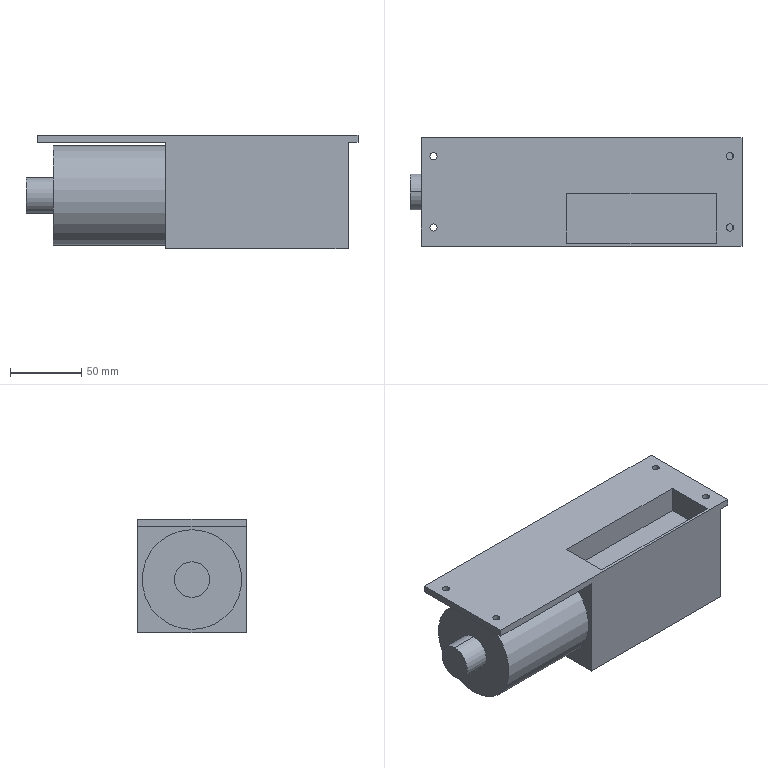Part | 1 solid | 33 faces | box 233 x 76 x 80 mm | volume 1016189 mm3 | plane 21 | cylinder 12 | commonest cylinder face diameters 5 x8 25 x2 70 x2
STEP:
#1=CARTESIAN_POINT('',(-120.5,0.,50.));
#2=VERTEX_POINT('',#1);
#3=CARTESIAN_POINT('',(-120.5,0.,25.));
#4=VERTEX_POINT('',#3);
#5=CARTESIAN_POINT('',(-120.5,0.,37.5));
#6=DIRECTION('',(-1.,0.,0.));
#7=DIRECTION('',(0.,0.,1.));
#8=AXIS2_PLACEMENT_3D('',#5,#6,#7);
#9=CIRCLE('',#8,12.5);
#10=EDGE_CURVE('',#2,#4,#9,.T.);
#11=ORIENTED_EDGE('',*,*,#10,.F.);
#12=CARTESIAN_POINT('',(-101.5,0.,50.));
#13=VERTEX_POINT('',#12);
#14=CARTESIAN_POINT('',(-120.5,0.,50.));
#15=DIRECTION('',(1.,0.,0.));
#16=VECTOR('',#15,1000.);
#17=LINE('',#14,#16);
#18=EDGE_CURVE('',#2,#13,#17,.T.);
#19=ORIENTED_EDGE('',*,*,#18,.T.);
#20=CARTESIAN_POINT('',(-101.5,0.,25.));
#21=VERTEX_POINT('',#20);
#22=CARTESIAN_POINT('',(-101.5,0.,37.5));
#23=DIRECTION('',(-1.,0.,0.));
#24=DIRECTION('',(0.,0.,1.));
#25=AXIS2_PLACEMENT_3D('',#22,#23,#24);
#26=CIRCLE('',#25,12.5);
#27=EDGE_CURVE('',#13,#21,#26,.T.);
#28=ORIENTED_EDGE('',*,*,#27,.T.);
#29=CARTESIAN_POINT('',(-120.5,0.,25.));
#30=DIRECTION('',(1.,0.,0.));
#31=VECTOR('',#30,1000.);
#32=LINE('',#29,#31);
#33=EDGE_CURVE('',#4,#21,#32,.T.);
#34=ORIENTED_EDGE('',*,*,#33,.F.);
#35=EDGE_LOOP('',(#11,#19,#28,#34));
#36=FACE_OUTER_BOUND('',#35,.T.);
#37=CARTESIAN_POINT('',(-120.5,0.,37.5));
#38=DIRECTION('',(1.,0.,0.));
#39=DIRECTION('',(0.,0.,-1.));
#40=AXIS2_PLACEMENT_3D('',#37,#38,#39);
#41=CYLINDRICAL_SURFACE('',#40,12.5);
#42=ADVANCED_FACE('',(#36),#41,.T.);
#43=CARTESIAN_POINT('',(-101.5,0.,72.5));
#44=VERTEX_POINT('',#43);
#45=CARTESIAN_POINT('',(-101.5,0.,2.5));
#46=VERTEX_POINT('',#45);
#47=CARTESIAN_POINT('',(-101.5,0.,37.5));
#48=DIRECTION('',(-1.,0.,0.));
#49=DIRECTION('',(0.,0.,1.));
#50=AXIS2_PLACEMENT_3D('',#47,#48,#49);
#51=CIRCLE('',#50,35.);
#52=EDGE_CURVE('',#44,#46,#51,.T.);
#53=ORIENTED_EDGE('',*,*,#52,.F.);
#54=CARTESIAN_POINT('',(-22.5,0.,72.5));
#55=VERTEX_POINT('',#54);
#56=CARTESIAN_POINT('',(-101.5,0.,72.5));
#57=DIRECTION('',(1.,0.,0.));
#58=VECTOR('',#57,1000.);
#59=LINE('',#56,#58);
#60=EDGE_CURVE('',#44,#55,#59,.T.);
#61=ORIENTED_EDGE('',*,*,#60,.T.);
#62=CARTESIAN_POINT('',(-22.5,0.,2.5));
#63=VERTEX_POINT('',#62);
#64=CARTESIAN_POINT('',(-22.5,0.,37.5));
#65=DIRECTION('',(-1.,0.,0.));
#66=DIRECTION('',(0.,0.,-1.));
#67=AXIS2_PLACEMENT_3D('',#64,#65,#66);
#68=CIRCLE('',#67,35.);
#69=EDGE_CURVE('',#55,#63,#68,.T.);
#70=ORIENTED_EDGE('',*,*,#69,.T.);
#71=CARTESIAN_POINT('',(-101.5,0.,2.5));
#72=DIRECTION('',(1.,0.,0.));
#73=VECTOR('',#72,1000.);
#74=LINE('',#71,#73);
#75=EDGE_CURVE('',#46,#63,#74,.T.);
#76=ORIENTED_EDGE('',*,*,#75,.F.);
#77=EDGE_LOOP('',(#53,#61,#70,#76));
#78=FACE_OUTER_BOUND('',#77,.T.);
#79=CARTESIAN_POINT('',(-101.5,0.,37.5));
#80=DIRECTION('',(1.,0.,0.));
#81=DIRECTION('',(0.,0.,-1.));
#82=AXIS2_PLACEMENT_3D('',#79,#80,#81);
#83=CYLINDRICAL_SURFACE('',#82,35.);
#84=ADVANCED_FACE('',(#78),#83,.T.);
#85=CARTESIAN_POINT('',(-106.5,25.,80.));
#86=VERTEX_POINT('',#85);
#87=CARTESIAN_POINT('',(-101.5,25.,80.));
#88=VERTEX_POINT('',#87);
#89=CARTESIAN_POINT('',(-104.,25.,80.));
#90=DIRECTION('',(0.,0.,1.));
#91=DIRECTION('',(1.,0.,0.));
#92=AXIS2_PLACEMENT_3D('',#89,#90,#91);
#93=CIRCLE('',#92,2.5);
#94=EDGE_CURVE('',#86,#88,#93,.T.);
#95=ORIENTED_EDGE('',*,*,#94,.T.);
#96=CARTESIAN_POINT('',(-101.5,25.,75.));
#97=VERTEX_POINT('',#96);
#98=CARTESIAN_POINT('',(-101.5,25.,90.));
#99=DIRECTION('',(0.,0.,-1.));
#100=VECTOR('',#99,1000.);
#101=LINE('',#98,#100);
#102=EDGE_CURVE('',#88,#97,#101,.T.);
#103=ORIENTED_EDGE('',*,*,#102,.T.);
#104=CARTESIAN_POINT('',(-106.5,25.,75.));
#105=VERTEX_POINT('',#104);
#106=CARTESIAN_POINT('',(-104.,25.,75.));
#107=DIRECTION('',(0.,0.,-1.));
#108=DIRECTION('',(-1.,0.,0.));
#109=AXIS2_PLACEMENT_3D('',#106,#107,#108);
#110=CIRCLE('',#109,2.5);
#111=EDGE_CURVE('',#97,#105,#110,.T.);
#112=ORIENTED_EDGE('',*,*,#111,.T.);
#113=CARTESIAN_POINT('',(-106.5,25.,90.));
#114=DIRECTION('',(0.,0.,-1.));
#115=VECTOR('',#114,1000.);
#116=LINE('',#113,#115);
#117=EDGE_CURVE('',#86,#105,#116,.T.);
#118=ORIENTED_EDGE('',*,*,#117,.F.);
#119=EDGE_LOOP('',(#95,#103,#112,#118));
#120=FACE_OUTER_BOUND('',#119,.T.);
#121=CARTESIAN_POINT('',(-104.,25.,90.));
#122=DIRECTION('',(0.,0.,-1.));
#123=DIRECTION('',(-1.,0.,0.));
#124=AXIS2_PLACEMENT_3D('',#121,#122,#123);
#125=CYLINDRICAL_SURFACE('',#124,2.5);
#126=ADVANCED_FACE('',(#120),#125,.F.);
#127=CARTESIAN_POINT('',(-106.5,-25.,80.));
#128=VERTEX_POINT('',#127);
#129=CARTESIAN_POINT('',(-101.5,-25.,80.));
#130=VERTEX_POINT('',#129);
#131=CARTESIAN_POINT('',(-104.,-25.,80.));
#132=DIRECTION('',(0.,0.,1.));
#133=DIRECTION('',(1.,0.,0.));
#134=AXIS2_PLACEMENT_3D('',#131,#132,#133);
#135=CIRCLE('',#134,2.5);
#136=EDGE_CURVE('',#128,#130,#135,.T.);
#137=ORIENTED_EDGE('',*,*,#136,.T.);
#138=CARTESIAN_POINT('',(-101.5,-25.,75.));
#139=VERTEX_POINT('',#138);
#140=CARTESIAN_POINT('',(-101.5,-25.,90.));
#141=DIRECTION('',(0.,0.,-1.));
#142=VECTOR('',#141,1000.);
#143=LINE('',#140,#142);
#144=EDGE_CURVE('',#130,#139,#143,.T.);
#145=ORIENTED_EDGE('',*,*,#144,.T.);
#146=CARTESIAN_POINT('',(-106.5,-25.,75.));
#147=VERTEX_POINT('',#146);
#148=CARTESIAN_POINT('',(-104.,-25.,75.));
#149=DIRECTION('',(0.,0.,-1.));
#150=DIRECTION('',(-1.,0.,0.));
#151=AXIS2_PLACEMENT_3D('',#148,#149,#150);
#152=CIRCLE('',#151,2.5);
#153=EDGE_CURVE('',#139,#147,#152,.T.);
#154=ORIENTED_EDGE('',*,*,#153,.T.);
#155=CARTESIAN_POINT('',(-106.5,-25.,90.));
#156=DIRECTION('',(0.,0.,-1.));
#157=VECTOR('',#156,1000.);
#158=LINE('',#155,#157);
#159=EDGE_CURVE('',#128,#147,#158,.T.);
#160=ORIENTED_EDGE('',*,*,#159,.F.);
#161=EDGE_LOOP('',(#137,#145,#154,#160));
#162=FACE_OUTER_BOUND('',#161,.T.);
#163=CARTESIAN_POINT('',(-104.,-25.,90.));
#164=DIRECTION('',(0.,0.,-1.));
#165=DIRECTION('',(-1.,0.,0.));
#166=AXIS2_PLACEMENT_3D('',#163,#164,#165);
#167=CYLINDRICAL_SURFACE('',#166,2.5);
#168=ADVANCED_FACE('',(#162),#167,.F.);
#169=CARTESIAN_POINT('',(101.5,-25.,80.));
#170=VERTEX_POINT('',#169);
#171=CARTESIAN_POINT('',(106.5,-25.,80.));
#172=VERTEX_POINT('',#171);
#173=CARTESIAN_POINT('',(104.,-25.,80.));
#174=DIRECTION('',(0.,0.,1.));
#175=DIRECTION('',(1.,0.,0.));
#176=AXIS2_PLACEMENT_3D('',#173,#174,#175);
#177=CIRCLE('',#176,2.5);
#178=EDGE_CURVE('',#170,#172,#177,.T.);
#179=ORIENTED_EDGE('',*,*,#178,.T.);
#180=CARTESIAN_POINT('',(106.5,-25.,75.));
#181=VERTEX_POINT('',#180);
#182=CARTESIAN_POINT('',(106.5,-25.,90.));
#183=DIRECTION('',(0.,0.,-1.));
#184=VECTOR('',#183,1000.);
#185=LINE('',#182,#184);
#186=EDGE_CURVE('',#172,#181,#185,.T.);
#187=ORIENTED_EDGE('',*,*,#186,.T.);
#188=CARTESIAN_POINT('',(101.5,-25.,75.));
#189=VERTEX_POINT('',#188);
#190=CARTESIAN_POINT('',(104.,-25.,75.));
#191=DIRECTION('',(0.,0.,-1.));
#192=DIRECTION('',(-1.,0.,0.));
#193=AXIS2_PLACEMENT_3D('',#190,#191,#192);
#194=CIRCLE('',#193,2.5);
#195=EDGE_CURVE('',#181,#189,#194,.T.);
#196=ORIENTED_EDGE('',*,*,#195,.T.);
#197=CARTESIAN_POINT('',(101.5,-25.,90.));
#198=DIRECTION('',(0.,0.,-1.));
#199=VECTOR('',#198,1000.);
#200=LINE('',#197,#199);
#201=EDGE_CURVE('',#170,#189,#200,.T.);
#202=ORIENTED_EDGE('',*,*,#201,.F.);
#203=EDGE_LOOP('',(#179,#187,#196,#202));
#204=FACE_OUTER_BOUND('',#203,.T.);
#205=CARTESIAN_POINT('',(104.,-25.,90.));
#206=DIRECTION('',(0.,0.,-1.));
#207=DIRECTION('',(-1.,0.,0.));
#208=AXIS2_PLACEMENT_3D('',#205,#206,#207);
#209=CYLINDRICAL_SURFACE('',#208,2.5);
#210=ADVANCED_FACE('',(#204),#209,.F.);
#211=CARTESIAN_POINT('',(101.5,25.,80.));
#212=VERTEX_POINT('',#211);
#213=CARTESIAN_POINT('',(106.5,25.,80.));
#214=VERTEX_POINT('',#213);
#215=CARTESIAN_POINT('',(104.,25.,80.));
#216=DIRECTION('',(0.,0.,1.));
#217=DIRECTION('',(1.,0.,0.));
#218=AXIS2_PLACEMENT_3D('',#215,#216,#217);
#219=CIRCLE('',#218,2.5);
#220=EDGE_CURVE('',#212,#214,#219,.T.);
#221=ORIENTED_EDGE('',*,*,#220,.T.);
#222=CARTESIAN_POINT('',(106.5,25.,75.));
#223=VERTEX_POINT('',#222);
#224=CARTESIAN_POINT('',(106.5,25.,90.));
#225=DIRECTION('',(0.,0.,-1.));
#226=VECTOR('',#225,1000.);
#227=LINE('',#224,#226);
#228=EDGE_CURVE('',#214,#223,#227,.T.);
#229=ORIENTED_EDGE('',*,*,#228,.T.);
#230=CARTESIAN_POINT('',(101.5,25.,75.));
#231=VERTEX_POINT('',#230);
#232=CARTESIAN_POINT('',(104.,25.,75.));
#233=DIRECTION('',(0.,0.,-1.));
#234=DIRECTION('',(-1.,0.,0.));
#235=AXIS2_PLACEMENT_3D('',#232,#233,#234);
#236=CIRCLE('',#235,2.5);
#237=EDGE_CURVE('',#223,#231,#236,.T.);
#238=ORIENTED_EDGE('',*,*,#237,.T.);
#239=CARTESIAN_POINT('',(101.5,25.,90.));
#240=DIRECTION('',(0.,0.,-1.));
#241=VECTOR('',#240,1000.);
#242=LINE('',#239,#241);
#243=EDGE_CURVE('',#212,#231,#242,.T.);
#244=ORIENTED_EDGE('',*,*,#243,.F.);
#245=EDGE_LOOP('',(#221,#229,#238,#244));
#246=FACE_OUTER_BOUND('',#245,.T.);
#247=CARTESIAN_POINT('',(104.,25.,90.));
#248=DIRECTION('',(0.,0.,-1.));
#249=DIRECTION('',(-1.,0.,0.));
#250=AXIS2_PLACEMENT_3D('',#247,#248,#249);
#251=CYLINDRICAL_SURFACE('',#250,2.5);
#252=ADVANCED_FACE('',(#246),#251,.F.);
#253=CARTESIAN_POINT('',(104.,-25.,75.));
#254=DIRECTION('',(0.,0.,-1.));
#255=DIRECTION('',(-1.,0.,0.));
#256=AXIS2_PLACEMENT_3D('',#253,#254,#255);
#257=CIRCLE('',#256,2.5);
#258=EDGE_CURVE('',#189,#181,#257,.T.);
#259=ORIENTED_EDGE('',*,*,#258,.F.);
#260=ORIENTED_EDGE('',*,*,#195,.F.);
#261=EDGE_LOOP('',(#259,#260));
#262=FACE_BOUND('',#261,.T.);
#263=CARTESIAN_POINT('',(104.,25.,75.));
#264=DIRECTION('',(0.,0.,-1.));
#265=DIRECTION('',(-1.,0.,0.));
#266=AXIS2_PLACEMENT_3D('',#263,#264,#265);
#267=CIRCLE('',#266,2.5);
#268=EDGE_CURVE('',#231,#223,#267,.T.);
#269=ORIENTED_EDGE('',*,*,#268,.F.);
#270=ORIENTED_EDGE('',*,*,#237,.F.);
#271=EDGE_LOOP('',(#269,#270));
#272=FACE_BOUND('',#271,.T.);
#273=CARTESIAN_POINT('',(105.5,-36.,75.));
#274=VERTEX_POINT('',#273);
#275=CARTESIAN_POINT('',(97.5,-36.,75.));
#276=VERTEX_POINT('',#275);
#277=CARTESIAN_POINT('',(105.5,-36.,75.));
#278=DIRECTION('',(-1.,0.,0.));
#279=VECTOR('',#278,1000.);
#280=LINE('',#277,#279);
#281=EDGE_CURVE('',#274,#276,#280,.T.);
#282=ORIENTED_EDGE('',*,*,#281,.T.);
#283=CARTESIAN_POINT('',(97.5,36.,75.));
#284=VERTEX_POINT('',#283);
#285=CARTESIAN_POINT('',(97.5,38.,75.));
#286=DIRECTION('',(0.,-1.,0.));
#287=VECTOR('',#286,1000.);
#288=LINE('',#285,#287);
#289=EDGE_CURVE('',#284,#276,#288,.T.);
#290=ORIENTED_EDGE('',*,*,#289,.F.);
#291=CARTESIAN_POINT('',(105.5,36.,75.));
#292=VERTEX_POINT('',#291);
#293=CARTESIAN_POINT('',(105.5,36.,75.));
#294=DIRECTION('',(-1.,0.,0.));
#295=VECTOR('',#294,1000.);
#296=LINE('',#293,#295);
#297=EDGE_CURVE('',#292,#284,#296,.T.);
#298=ORIENTED_EDGE('',*,*,#297,.F.);
#299=CARTESIAN_POINT('',(105.5,38.,75.));
#300=VERTEX_POINT('',#299);
#301=CARTESIAN_POINT('',(105.5,38.,75.));
#302=DIRECTION('',(0.,-1.,0.));
#303=VECTOR('',#302,1000.);
#304=LINE('',#301,#303);
#305=EDGE_CURVE('',#300,#292,#304,.T.);
#306=ORIENTED_EDGE('',*,*,#305,.F.);
#307=CARTESIAN_POINT('',(112.5,38.,75.));
#308=VERTEX_POINT('',#307);
#309=CARTESIAN_POINT('',(97.5,38.,75.));
#310=DIRECTION('',(1.,0.,0.));
#311=VECTOR('',#310,1000.);
#312=LINE('',#309,#311);
#313=EDGE_CURVE('',#300,#308,#312,.T.);
#314=ORIENTED_EDGE('',*,*,#313,.T.);
#315=CARTESIAN_POINT('',(112.5,-38.,75.));
#316=VERTEX_POINT('',#315);
#317=CARTESIAN_POINT('',(112.5,38.,75.));
#318=DIRECTION('',(0.,-1.,0.));
#319=VECTOR('',#318,1000.);
#320=LINE('',#317,#319);
#321=EDGE_CURVE('',#308,#316,#320,.T.);
#322=ORIENTED_EDGE('',*,*,#321,.T.);
#323=CARTESIAN_POINT('',(105.5,-38.,75.));
#324=VERTEX_POINT('',#323);
#325=CARTESIAN_POINT('',(97.5,-38.,75.));
#326=DIRECTION('',(1.,0.,0.));
#327=VECTOR('',#326,1000.);
#328=LINE('',#325,#327);
#329=EDGE_CURVE('',#324,#316,#328,.T.);
#330=ORIENTED_EDGE('',*,*,#329,.F.);
#331=CARTESIAN_POINT('',(105.5,-38.,75.));
#332=DIRECTION('',(0.,-1.,0.));
#333=VECTOR('',#332,1000.);
#334=LINE('',#331,#333);
#335=EDGE_CURVE('',#274,#324,#334,.T.);
#336=ORIENTED_EDGE('',*,*,#335,.F.);
#337=EDGE_LOOP('',(#282,#290,#298,#306,#314,#322,#330,#336));
#338=FACE_OUTER_BOUND('',#337,.T.);
#339=CARTESIAN_POINT('',(97.5,38.,75.));
#340=DIRECTION('',(0.,0.,1.));
#341=DIRECTION('',(0.,-1.,0.));
#342=AXIS2_PLACEMENT_3D('',#339,#340,#341);
#343=PLANE('',#342);
#344=ADVANCED_FACE('',(#262,#272,#338),#343,.F.);
#345=CARTESIAN_POINT('',(97.5,36.,2.));
#346=VERTEX_POINT('',#345);
#347=CARTESIAN_POINT('',(97.5,36.,75.));
#348=DIRECTION('',(0.,0.,-1.));
#349=VECTOR('',#348,1000.);
#350=LINE('',#347,#349);
#351=EDGE_CURVE('',#284,#346,#350,.T.);
#352=ORIENTED_EDGE('',*,*,#351,.F.);
#353=ORIENTED_EDGE('',*,*,#289,.T.);
#354=CARTESIAN_POINT('',(97.5,-36.,2.));
#355=VERTEX_POINT('',#354);
#356=CARTESIAN_POINT('',(97.5,-36.,75.));
#357=DIRECTION('',(0.,0.,1.));
#358=VECTOR('',#357,1000.);
#359=LINE('',#356,#358);
#360=EDGE_CURVE('',#355,#276,#359,.T.);
#361=ORIENTED_EDGE('',*,*,#360,.F.);
#362=CARTESIAN_POINT('',(97.5,36.,2.));
#363=DIRECTION('',(0.,-1.,0.));
#364=VECTOR('',#363,1000.);
#365=LINE('',#362,#364);
#366=EDGE_CURVE('',#346,#355,#365,.T.);
#367=ORIENTED_EDGE('',*,*,#366,.F.);
#368=EDGE_LOOP('',(#352,#353,#361,#367));
#369=FACE_OUTER_BOUND('',#368,.T.);
#370=CARTESIAN_POINT('',(97.5,0.,0.));
#371=DIRECTION('',(-1.,0.,0.));
#372=DIRECTION('',(0.,-1.,0.));
#373=AXIS2_PLACEMENT_3D('',#370,#371,#372);
#374=PLANE('',#373);
#375=ADVANCED_FACE('',(#369),#374,.F.);
#376=CARTESIAN_POINT('',(112.5,-38.,80.));
#377=VERTEX_POINT('',#376);
#378=CARTESIAN_POINT('',(112.5,-38.,80.));
#379=DIRECTION('',(0.,0.,-1.));
#380=VECTOR('',#379,1000.);
#381=LINE('',#378,#380);
#382=EDGE_CURVE('',#377,#316,#381,.T.);
#383=ORIENTED_EDGE('',*,*,#382,.T.);
#384=ORIENTED_EDGE('',*,*,#321,.F.);
#385=CARTESIAN_POINT('',(112.5,38.,80.));
#386=VERTEX_POINT('',#385);
#387=CARTESIAN_POINT('',(112.5,38.,80.));
#388=DIRECTION('',(0.,0.,-1.));
#389=VECTOR('',#388,1000.);
#390=LINE('',#387,#389);
#391=EDGE_CURVE('',#386,#308,#390,.T.);
#392=ORIENTED_EDGE('',*,*,#391,.F.);
#393=CARTESIAN_POINT('',(112.5,38.,80.));
#394=DIRECTION('',(0.,1.,0.));
#395=VECTOR('',#394,1000.);
#396=LINE('',#393,#395);
#397=EDGE_CURVE('',#377,#386,#396,.T.);
#398=ORIENTED_EDGE('',*,*,#397,.F.);
#399=EDGE_LOOP('',(#383,#384,#392,#398));
#400=FACE_OUTER_BOUND('',#399,.T.);
#401=CARTESIAN_POINT('',(112.5,38.,80.));
#402=DIRECTION('',(-1.,0.,0.));
#403=DIRECTION('',(0.,-1.,0.));
#404=AXIS2_PLACEMENT_3D('',#401,#402,#403);
#405=PLANE('',#404);
#406=ADVANCED_FACE('',(#400),#405,.F.);
#407=ORIENTED_EDGE('',*,*,#313,.F.);
#408=CARTESIAN_POINT('',(105.5,38.,0.));
#409=VERTEX_POINT('',#408);
#410=CARTESIAN_POINT('',(105.5,38.,75.));
#411=DIRECTION('',(0.,0.,1.));
#412=VECTOR('',#411,1000.);
#413=LINE('',#410,#412);
#414=EDGE_CURVE('',#409,#300,#413,.T.);
#415=ORIENTED_EDGE('',*,*,#414,.F.);
#416=CARTESIAN_POINT('',(-22.5,38.,0.));
#417=VERTEX_POINT('',#416);
#418=CARTESIAN_POINT('',(-112.5,38.,0.));
#419=DIRECTION('',(-1.,0.,0.));
#420=VECTOR('',#419,1000.);
#421=LINE('',#418,#420);
#422=EDGE_CURVE('',#409,#417,#421,.T.);
#423=ORIENTED_EDGE('',*,*,#422,.T.);
#424=CARTESIAN_POINT('',(-22.5,38.,75.));
#425=VERTEX_POINT('',#424);
#426=CARTESIAN_POINT('',(-22.5,38.,0.));
#427=DIRECTION('',(0.,0.,-1.));
#428=VECTOR('',#427,1000.);
#429=LINE('',#426,#428);
#430=EDGE_CURVE('',#425,#417,#429,.T.);
#431=ORIENTED_EDGE('',*,*,#430,.F.);
#432=CARTESIAN_POINT('',(-112.5,38.,75.));
#433=VERTEX_POINT('',#432);
#434=CARTESIAN_POINT('',(-22.5,38.,75.));
#435=DIRECTION('',(-1.,0.,0.));
#436=VECTOR('',#435,1000.);
#437=LINE('',#434,#436);
#438=EDGE_CURVE('',#425,#433,#437,.T.);
#439=ORIENTED_EDGE('',*,*,#438,.T.);
#440=CARTESIAN_POINT('',(-112.5,38.,80.));
#441=VERTEX_POINT('',#440);
#442=CARTESIAN_POINT('',(-112.5,38.,80.));
#443=DIRECTION('',(0.,0.,-1.));
#444=VECTOR('',#443,1000.);
#445=LINE('',#442,#444);
#446=EDGE_CURVE('',#441,#433,#445,.T.);
#447=ORIENTED_EDGE('',*,*,#446,.F.);
#448=CARTESIAN_POINT('',(-112.5,38.,80.));
#449=DIRECTION('',(-1.,0.,0.));
#450=VECTOR('',#449,1000.);
#451=LINE('',#448,#450);
#452=EDGE_CURVE('',#386,#441,#451,.T.);
#453=ORIENTED_EDGE('',*,*,#452,.F.);
#454=ORIENTED_EDGE('',*,*,#391,.T.);
#455=EDGE_LOOP('',(#407,#415,#423,#431,#439,#447,#453,#454));
#456=FACE_OUTER_BOUND('',#455,.T.);
#457=CARTESIAN_POINT('',(-112.5,38.,80.));
#458=DIRECTION('',(0.,-1.,0.));
#459=DIRECTION('',(0.,0.,-1.));
#460=AXIS2_PLACEMENT_3D('',#457,#458,#459);
#461=PLANE('',#460);
#462=ADVANCED_FACE('',(#456),#461,.F.);
#463=ORIENTED_EDGE('',*,*,#446,.T.);
#464=CARTESIAN_POINT('',(-112.5,-38.,75.));
#465=VERTEX_POINT('',#464);
#466=CARTESIAN_POINT('',(-112.5,-38.,75.));
#467=DIRECTION('',(0.,1.,0.));
#468=VECTOR('',#467,1000.);
#469=LINE('',#466,#468);
#470=EDGE_CURVE('',#465,#433,#469,.T.);
#471=ORIENTED_EDGE('',*,*,#470,.F.);
#472=CARTESIAN_POINT('',(-112.5,-38.,80.));
#473=VERTEX_POINT('',#472);
#474=CARTESIAN_POINT('',(-112.5,-38.,80.));
#475=DIRECTION('',(0.,0.,-1.));
#476=VECTOR('',#475,1000.);
#477=LINE('',#474,#476);
#478=EDGE_CURVE('',#473,#465,#477,.T.);
#479=ORIENTED_EDGE('',*,*,#478,.F.);
#480=CARTESIAN_POINT('',(-112.5,38.,80.));
#481=DIRECTION('',(0.,-1.,0.));
#482=VECTOR('',#481,1000.);
#483=LINE('',#480,#482);
#484=EDGE_CURVE('',#441,#473,#483,.T.);
#485=ORIENTED_EDGE('',*,*,#484,.F.);
#486=EDGE_LOOP('',(#463,#471,#479,#485));
#487=FACE_OUTER_BOUND('',#486,.T.);
#488=CARTESIAN_POINT('',(-112.5,38.,80.));
#489=DIRECTION('',(1.,0.,0.));
#490=DIRECTION('',(0.,0.,-1.));
#491=AXIS2_PLACEMENT_3D('',#488,#489,#490);
#492=PLANE('',#491);
#493=ADVANCED_FACE('',(#487),#492,.F.);
#494=CARTESIAN_POINT('',(105.5,-38.,0.));
#495=VERTEX_POINT('',#494);
#496=CARTESIAN_POINT('',(105.5,-38.,0.));
#497=DIRECTION('',(0.,0.,-1.));
#498=VECTOR('',#497,1000.);
#499=LINE('',#496,#498);
#500=EDGE_CURVE('',#324,#495,#499,.T.);
#501=ORIENTED_EDGE('',*,*,#500,.F.);
#502=ORIENTED_EDGE('',*,*,#329,.T.);
#503=ORIENTED_EDGE('',*,*,#382,.F.);
#504=CARTESIAN_POINT('',(-112.5,-38.,80.));
#505=DIRECTION('',(1.,0.,0.));
#506=VECTOR('',#505,1000.);
#507=LINE('',#504,#506);
#508=EDGE_CURVE('',#473,#377,#507,.T.);
#509=ORIENTED_EDGE('',*,*,#508,.F.);
#510=ORIENTED_EDGE('',*,*,#478,.T.);
#511=CARTESIAN_POINT('',(-22.5,-38.,75.));
#512=VERTEX_POINT('',#511);
#513=CARTESIAN_POINT('',(-22.5,-38.,75.));
#514=DIRECTION('',(-1.,0.,0.));
#515=VECTOR('',#514,1000.);
#516=LINE('',#513,#515);
#517=EDGE_CURVE('',#512,#465,#516,.T.);
#518=ORIENTED_EDGE('',*,*,#517,.F.);
#519=CARTESIAN_POINT('',(-22.5,-38.,0.));
#520=VERTEX_POINT('',#519);
#521=CARTESIAN_POINT('',(-22.5,-38.,0.));
#522=DIRECTION('',(0.,0.,1.));
#523=VECTOR('',#522,1000.);
#524=LINE('',#521,#523);
#525=EDGE_CURVE('',#520,#512,#524,.T.);
#526=ORIENTED_EDGE('',*,*,#525,.F.);
#527=CARTESIAN_POINT('',(-112.5,-38.,0.));
#528=DIRECTION('',(1.,0.,0.));
#529=VECTOR('',#528,1000.);
#530=LINE('',#527,#529);
#531=EDGE_CURVE('',#520,#495,#530,.T.);
#532=ORIENTED_EDGE('',*,*,#531,.T.);
#533=EDGE_LOOP('',(#501,#502,#503,#509,#510,#518,#526,#532));
#534=FACE_OUTER_BOUND('',#533,.T.);
#535=CARTESIAN_POINT('',(-112.5,-38.,80.));
#536=DIRECTION('',(0.,1.,0.));
#537=DIRECTION('',(0.,0.,1.));
#538=AXIS2_PLACEMENT_3D('',#535,#536,#537);
#539=PLANE('',#538);
#540=ADVANCED_FACE('',(#534),#539,.F.);
#541=CARTESIAN_POINT('',(-10.5,-1.,80.));
#542=VERTEX_POINT('',#541);
#543=CARTESIAN_POINT('',(-10.5,-36.,80.));
#544=VERTEX_POINT('',#543);
#545=CARTESIAN_POINT('',(-10.5,-1.,80.));
#546=DIRECTION('',(0.,-1.,0.));
#547=VECTOR('',#546,1000.);
#548=LINE('',#545,#547);
#549=EDGE_CURVE('',#542,#544,#548,.T.);
#550=ORIENTED_EDGE('',*,*,#549,.F.);
#551=CARTESIAN_POINT('',(94.5,-1.,80.));
#552=VERTEX_POINT('',#551);
#553=CARTESIAN_POINT('',(-10.5,-1.,80.));
#554=DIRECTION('',(-1.,0.,0.));
#555=VECTOR('',#554,1000.);
#556=LINE('',#553,#555);
#557=EDGE_CURVE('',#552,#542,#556,.T.);
#558=ORIENTED_EDGE('',*,*,#557,.F.);
#559=CARTESIAN_POINT('',(94.5,-36.,80.));
#560=VERTEX_POINT('',#559);
#561=CARTESIAN_POINT('',(94.5,-1.,80.));
#562=DIRECTION('',(0.,1.,0.));
#563=VECTOR('',#562,1000.);
#564=LINE('',#561,#563);
#565=EDGE_CURVE('',#560,#552,#564,.T.);
#566=ORIENTED_EDGE('',*,*,#565,.F.);
#567=CARTESIAN_POINT('',(-10.5,-36.,80.));
#568=DIRECTION('',(1.,0.,0.));
#569=VECTOR('',#568,1000.);
#570=LINE('',#567,#569);
#571=EDGE_CURVE('',#544,#560,#570,.T.);
#572=ORIENTED_EDGE('',*,*,#571,.F.);
#573=EDGE_LOOP('',(#550,#558,#566,#572));
#574=FACE_BOUND('',#573,.T.);
#575=ORIENTED_EDGE('',*,*,#94,.F.);
#576=CARTESIAN_POINT('',(-104.,25.,80.));
#577=DIRECTION('',(0.,0.,1.));
#578=DIRECTION('',(1.,0.,0.));
#579=AXIS2_PLACEMENT_3D('',#576,#577,#578);
#580=CIRCLE('',#579,2.5);
#581=EDGE_CURVE('',#88,#86,#580,.T.);
#582=ORIENTED_EDGE('',*,*,#581,.F.);
#583=EDGE_LOOP('',(#575,#582));
#584=FACE_BOUND('',#583,.T.);
#585=ORIENTED_EDGE('',*,*,#178,.F.);
#586=CARTESIAN_POINT('',(104.,-25.,80.));
#587=DIRECTION('',(0.,0.,1.));
#588=DIRECTION('',(1.,0.,0.));
#589=AXIS2_PLACEMENT_3D('',#586,#587,#588);
#590=CIRCLE('',#589,2.5);
#591=EDGE_CURVE('',#172,#170,#590,.T.);
#592=ORIENTED_EDGE('',*,*,#591,.F.);
#593=EDGE_LOOP('',(#585,#592));
#594=FACE_BOUND('',#593,.T.);
#595=ORIENTED_EDGE('',*,*,#220,.F.);
#596=CARTESIAN_POINT('',(104.,25.,80.));
#597=DIRECTION('',(0.,0.,1.));
#598=DIRECTION('',(1.,0.,0.));
#599=AXIS2_PLACEMENT_3D('',#596,#597,#598);
#600=CIRCLE('',#599,2.5);
#601=EDGE_CURVE('',#214,#212,#600,.T.);
#602=ORIENTED_EDGE('',*,*,#601,.F.);
#603=EDGE_LOOP('',(#595,#602));
#604=FACE_BOUND('',#603,.T.);
#605=ORIENTED_EDGE('',*,*,#136,.F.);
#606=CARTESIAN_POINT('',(-104.,-25.,80.));
#607=DIRECTION('',(0.,0.,1.));
#608=DIRECTION('',(1.,0.,0.));
#609=AXIS2_PLACEMENT_3D('',#606,#607,#608);
#610=CIRCLE('',#609,2.5);
#611=EDGE_CURVE('',#130,#128,#610,.T.);
#612=ORIENTED_EDGE('',*,*,#611,.F.);
#613=EDGE_LOOP('',(#605,#612));
#614=FACE_BOUND('',#613,.T.);
#615=ORIENTED_EDGE('',*,*,#397,.T.);
#616=ORIENTED_EDGE('',*,*,#452,.T.);
#617=ORIENTED_EDGE('',*,*,#484,.T.);
#618=ORIENTED_EDGE('',*,*,#508,.T.);
#619=EDGE_LOOP('',(#615,#616,#617,#618));
#620=FACE_OUTER_BOUND('',#619,.T.);
#621=CARTESIAN_POINT('',(0.,0.,80.));
#622=DIRECTION('',(0.,0.,1.));
#623=DIRECTION('',(1.,0.,0.));
#624=AXIS2_PLACEMENT_3D('',#621,#622,#623);
#625=PLANE('',#624);
#626=ADVANCED_FACE('',(#574,#584,#594,#604,#614,#620),#625,.T.);
#627=ORIENTED_EDGE('',*,*,#422,.F.);
#628=CARTESIAN_POINT('',(105.5,38.,0.));
#629=DIRECTION('',(0.,1.,0.));
#630=VECTOR('',#629,1000.);
#631=LINE('',#628,#630);
#632=EDGE_CURVE('',#495,#409,#631,.T.);
#633=ORIENTED_EDGE('',*,*,#632,.F.);
#634=ORIENTED_EDGE('',*,*,#531,.F.);
#635=CARTESIAN_POINT('',(-22.5,-38.,0.));
#636=DIRECTION('',(0.,-1.,0.));
#637=VECTOR('',#636,1000.);
#638=LINE('',#635,#637);
#639=EDGE_CURVE('',#417,#520,#638,.T.);
#640=ORIENTED_EDGE('',*,*,#639,.F.);
#641=EDGE_LOOP('',(#627,#633,#634,#640));
#642=FACE_OUTER_BOUND('',#641,.T.);
#643=CARTESIAN_POINT('',(0.,0.,0.));
#644=DIRECTION('',(0.,0.,1.));
#645=DIRECTION('',(1.,0.,0.));
#646=AXIS2_PLACEMENT_3D('',#643,#644,#645);
#647=PLANE('',#646);
#648=ADVANCED_FACE('',(#642),#647,.F.);
#649=CARTESIAN_POINT('',(-104.,25.,75.));
#650=DIRECTION('',(0.,0.,-1.));
#651=DIRECTION('',(-1.,0.,0.));
#652=AXIS2_PLACEMENT_3D('',#649,#650,#651);
#653=CIRCLE('',#652,2.5);
#654=EDGE_CURVE('',#105,#97,#653,.T.);
#655=ORIENTED_EDGE('',*,*,#654,.F.);
#656=ORIENTED_EDGE('',*,*,#111,.F.);
#657=EDGE_LOOP('',(#655,#656));
#658=FACE_BOUND('',#657,.T.);
#659=CARTESIAN_POINT('',(-104.,-25.,75.));
#660=DIRECTION('',(0.,0.,-1.));
#661=DIRECTION('',(-1.,0.,0.));
#662=AXIS2_PLACEMENT_3D('',#659,#660,#661);
#663=CIRCLE('',#662,2.5);
#664=EDGE_CURVE('',#147,#139,#663,.T.);
#665=ORIENTED_EDGE('',*,*,#664,.F.);
#666=ORIENTED_EDGE('',*,*,#153,.F.);
#667=EDGE_LOOP('',(#665,#666));
#668=FACE_BOUND('',#667,.T.);
#669=ORIENTED_EDGE('',*,*,#470,.T.);
#670=ORIENTED_EDGE('',*,*,#438,.F.);
#671=CARTESIAN_POINT('',(-22.5,-38.,75.));
#672=DIRECTION('',(0.,1.,0.));
#673=VECTOR('',#672,1000.);
#674=LINE('',#671,#673);
#675=EDGE_CURVE('',#512,#425,#674,.T.);
#676=ORIENTED_EDGE('',*,*,#675,.F.);
#677=ORIENTED_EDGE('',*,*,#517,.T.);
#678=EDGE_LOOP('',(#669,#670,#676,#677));
#679=FACE_OUTER_BOUND('',#678,.T.);
#680=CARTESIAN_POINT('',(-22.5,-38.,75.));
#681=DIRECTION('',(0.,0.,1.));
#682=DIRECTION('',(1.,0.,0.));
#683=AXIS2_PLACEMENT_3D('',#680,#681,#682);
#684=PLANE('',#683);
#685=ADVANCED_FACE('',(#658,#668,#679),#684,.F.);
#686=CARTESIAN_POINT('',(-22.5,0.,37.5));
#687=DIRECTION('',(-1.,0.,0.));
#688=DIRECTION('',(0.,0.,-1.));
#689=AXIS2_PLACEMENT_3D('',#686,#687,#688);
#690=CIRCLE('',#689,35.);
#691=EDGE_CURVE('',#63,#55,#690,.T.);
#692=ORIENTED_EDGE('',*,*,#691,.F.);
#693=ORIENTED_EDGE('',*,*,#69,.F.);
#694=EDGE_LOOP('',(#692,#693));
#695=FACE_BOUND('',#694,.T.);
#696=ORIENTED_EDGE('',*,*,#639,.T.);
#697=ORIENTED_EDGE('',*,*,#525,.T.);
#698=ORIENTED_EDGE('',*,*,#675,.T.);
#699=ORIENTED_EDGE('',*,*,#430,.T.);
#700=EDGE_LOOP('',(#696,#697,#698,#699));
#701=FACE_OUTER_BOUND('',#700,.T.);
#702=CARTESIAN_POINT('',(-22.5,0.,0.));
#703=DIRECTION('',(1.,0.,0.));
#704=DIRECTION('',(0.,0.,-1.));
#705=AXIS2_PLACEMENT_3D('',#702,#703,#704);
#706=PLANE('',#705);
#707=ADVANCED_FACE('',(#695,#701),#706,.F.);
#708=ORIENTED_EDGE('',*,*,#228,.F.);
#709=ORIENTED_EDGE('',*,*,#601,.T.);
#710=ORIENTED_EDGE('',*,*,#243,.T.);
#711=ORIENTED_EDGE('',*,*,#268,.T.);
#712=EDGE_LOOP('',(#708,#709,#710,#711));
#713=FACE_OUTER_BOUND('',#712,.T.);
#714=CARTESIAN_POINT('',(104.,25.,90.));
#715=DIRECTION('',(0.,0.,-1.));
#716=DIRECTION('',(-1.,0.,0.));
#717=AXIS2_PLACEMENT_3D('',#714,#715,#716);
#718=CYLINDRICAL_SURFACE('',#717,2.5);
#719=ADVANCED_FACE('',(#713),#718,.F.);
#720=ORIENTED_EDGE('',*,*,#186,.F.);
#721=ORIENTED_EDGE('',*,*,#591,.T.);
#722=ORIENTED_EDGE('',*,*,#201,.T.);
#723=ORIENTED_EDGE('',*,*,#258,.T.);
#724=EDGE_LOOP('',(#720,#721,#722,#723));
#725=FACE_OUTER_BOUND('',#724,.T.);
#726=CARTESIAN_POINT('',(104.,-25.,90.));
#727=DIRECTION('',(0.,0.,-1.));
#728=DIRECTION('',(-1.,0.,0.));
#729=AXIS2_PLACEMENT_3D('',#726,#727,#728);
#730=CYLINDRICAL_SURFACE('',#729,2.5);
#731=ADVANCED_FACE('',(#725),#730,.F.);
#732=ORIENTED_EDGE('',*,*,#144,.F.);
#733=ORIENTED_EDGE('',*,*,#611,.T.);
#734=ORIENTED_EDGE('',*,*,#159,.T.);
#735=ORIENTED_EDGE('',*,*,#664,.T.);
#736=EDGE_LOOP('',(#732,#733,#734,#735));
#737=FACE_OUTER_BOUND('',#736,.T.);
#738=CARTESIAN_POINT('',(-104.,-25.,90.));
#739=DIRECTION('',(0.,0.,-1.));
#740=DIRECTION('',(-1.,0.,0.));
#741=AXIS2_PLACEMENT_3D('',#738,#739,#740);
#742=CYLINDRICAL_SURFACE('',#741,2.5);
#743=ADVANCED_FACE('',(#737),#742,.F.);
#744=ORIENTED_EDGE('',*,*,#102,.F.);
#745=ORIENTED_EDGE('',*,*,#581,.T.);
#746=ORIENTED_EDGE('',*,*,#117,.T.);
#747=ORIENTED_EDGE('',*,*,#654,.T.);
#748=EDGE_LOOP('',(#744,#745,#746,#747));
#749=FACE_OUTER_BOUND('',#748,.T.);
#750=CARTESIAN_POINT('',(-104.,25.,90.));
#751=DIRECTION('',(0.,0.,-1.));
#752=DIRECTION('',(-1.,0.,0.));
#753=AXIS2_PLACEMENT_3D('',#750,#751,#752);
#754=CYLINDRICAL_SURFACE('',#753,2.5);
#755=ADVANCED_FACE('',(#749),#754,.F.);
#756=ORIENTED_EDGE('',*,*,#60,.F.);
#757=CARTESIAN_POINT('',(-101.5,0.,37.5));
#758=DIRECTION('',(-1.,0.,0.));
#759=DIRECTION('',(0.,0.,1.));
#760=AXIS2_PLACEMENT_3D('',#757,#758,#759);
#761=CIRCLE('',#760,35.);
#762=EDGE_CURVE('',#46,#44,#761,.T.);
#763=ORIENTED_EDGE('',*,*,#762,.F.);
#764=ORIENTED_EDGE('',*,*,#75,.T.);
#765=ORIENTED_EDGE('',*,*,#691,.T.);
#766=EDGE_LOOP('',(#756,#763,#764,#765));
#767=FACE_OUTER_BOUND('',#766,.T.);
#768=CARTESIAN_POINT('',(-101.5,0.,37.5));
#769=DIRECTION('',(1.,0.,0.));
#770=DIRECTION('',(0.,0.,-1.));
#771=AXIS2_PLACEMENT_3D('',#768,#769,#770);
#772=CYLINDRICAL_SURFACE('',#771,35.);
#773=ADVANCED_FACE('',(#767),#772,.T.);
#774=CARTESIAN_POINT('',(-101.5,0.,37.5));
#775=DIRECTION('',(-1.,0.,0.));
#776=DIRECTION('',(0.,0.,1.));
#777=AXIS2_PLACEMENT_3D('',#774,#775,#776);
#778=CIRCLE('',#777,12.5);
#779=EDGE_CURVE('',#21,#13,#778,.T.);
#780=ORIENTED_EDGE('',*,*,#779,.F.);
#781=ORIENTED_EDGE('',*,*,#27,.F.);
#782=EDGE_LOOP('',(#780,#781));
#783=FACE_BOUND('',#782,.T.);
#784=ORIENTED_EDGE('',*,*,#762,.T.);
#785=ORIENTED_EDGE('',*,*,#52,.T.);
#786=EDGE_LOOP('',(#784,#785));
#787=FACE_OUTER_BOUND('',#786,.T.);
#788=CARTESIAN_POINT('',(-101.5,0.,37.5));
#789=DIRECTION('',(-1.,0.,0.));
#790=DIRECTION('',(0.,0.,1.));
#791=AXIS2_PLACEMENT_3D('',#788,#789,#790);
#792=PLANE('',#791);
#793=ADVANCED_FACE('',(#783,#787),#792,.T.);
#794=ORIENTED_EDGE('',*,*,#18,.F.);
#795=CARTESIAN_POINT('',(-120.5,0.,37.5));
#796=DIRECTION('',(-1.,0.,0.));
#797=DIRECTION('',(0.,0.,1.));
#798=AXIS2_PLACEMENT_3D('',#795,#796,#797);
#799=CIRCLE('',#798,12.5);
#800=EDGE_CURVE('',#4,#2,#799,.T.);
#801=ORIENTED_EDGE('',*,*,#800,.F.);
#802=ORIENTED_EDGE('',*,*,#33,.T.);
#803=ORIENTED_EDGE('',*,*,#779,.T.);
#804=EDGE_LOOP('',(#794,#801,#802,#803));
#805=FACE_OUTER_BOUND('',#804,.T.);
#806=CARTESIAN_POINT('',(-120.5,0.,37.5));
#807=DIRECTION('',(1.,0.,0.));
#808=DIRECTION('',(0.,0.,-1.));
#809=AXIS2_PLACEMENT_3D('',#806,#807,#808);
#810=CYLINDRICAL_SURFACE('',#809,12.5);
#811=ADVANCED_FACE('',(#805),#810,.T.);
#812=ORIENTED_EDGE('',*,*,#800,.T.);
#813=ORIENTED_EDGE('',*,*,#10,.T.);
#814=EDGE_LOOP('',(#812,#813));
#815=FACE_OUTER_BOUND('',#814,.T.);
#816=CARTESIAN_POINT('',(-120.5,0.,37.5));
#817=DIRECTION('',(-1.,0.,0.));
#818=DIRECTION('',(0.,0.,1.));
#819=AXIS2_PLACEMENT_3D('',#816,#817,#818);
#820=PLANE('',#819);
#821=ADVANCED_FACE('',(#815),#820,.T.);
#822=ORIENTED_EDGE('',*,*,#549,.T.);
#823=CARTESIAN_POINT('',(-10.5,-36.,61.));
#824=VERTEX_POINT('',#823);
#825=CARTESIAN_POINT('',(-10.5,-36.,61.));
#826=DIRECTION('',(0.,0.,1.));
#827=VECTOR('',#826,1000.);
#828=LINE('',#825,#827);
#829=EDGE_CURVE('',#824,#544,#828,.T.);
#830=ORIENTED_EDGE('',*,*,#829,.F.);
#831=CARTESIAN_POINT('',(-10.5,-1.,61.));
#832=VERTEX_POINT('',#831);
#833=CARTESIAN_POINT('',(-10.5,-1.,61.));
#834=DIRECTION('',(0.,-1.,0.));
#835=VECTOR('',#834,1000.);
#836=LINE('',#833,#835);
#837=EDGE_CURVE('',#832,#824,#836,.T.);
#838=ORIENTED_EDGE('',*,*,#837,.F.);
#839=CARTESIAN_POINT('',(-10.5,-1.,61.));
#840=DIRECTION('',(0.,0.,1.));
#841=VECTOR('',#840,1000.);
#842=LINE('',#839,#841);
#843=EDGE_CURVE('',#832,#542,#842,.T.);
#844=ORIENTED_EDGE('',*,*,#843,.T.);
#845=EDGE_LOOP('',(#822,#830,#838,#844));
#846=FACE_OUTER_BOUND('',#845,.T.);
#847=CARTESIAN_POINT('',(-10.5,-1.,61.));
#848=DIRECTION('',(-1.,0.,0.));
#849=DIRECTION('',(0.,-1.,0.));
#850=AXIS2_PLACEMENT_3D('',#847,#848,#849);
#851=PLANE('',#850);
#852=ADVANCED_FACE('',(#846),#851,.F.);
#853=ORIENTED_EDGE('',*,*,#557,.T.);
#854=ORIENTED_EDGE('',*,*,#843,.F.);
#855=CARTESIAN_POINT('',(94.5,-1.,61.));
#856=VERTEX_POINT('',#855);
#857=CARTESIAN_POINT('',(-10.5,-1.,61.));
#858=DIRECTION('',(-1.,0.,0.));
#859=VECTOR('',#858,1000.);
#860=LINE('',#857,#859);
#861=EDGE_CURVE('',#856,#832,#860,.T.);
#862=ORIENTED_EDGE('',*,*,#861,.F.);
#863=CARTESIAN_POINT('',(94.5,-1.,61.));
#864=DIRECTION('',(0.,0.,1.));
#865=VECTOR('',#864,1000.);
#866=LINE('',#863,#865);
#867=EDGE_CURVE('',#856,#552,#866,.T.);
#868=ORIENTED_EDGE('',*,*,#867,.T.);
#869=EDGE_LOOP('',(#853,#854,#862,#868));
#870=FACE_OUTER_BOUND('',#869,.T.);
#871=CARTESIAN_POINT('',(-10.5,-1.,61.));
#872=DIRECTION('',(0.,1.,0.));
#873=DIRECTION('',(0.,0.,1.));
#874=AXIS2_PLACEMENT_3D('',#871,#872,#873);
#875=PLANE('',#874);
#876=ADVANCED_FACE('',(#870),#875,.F.);
#877=ORIENTED_EDGE('',*,*,#565,.T.);
#878=ORIENTED_EDGE('',*,*,#867,.F.);
#879=CARTESIAN_POINT('',(94.5,-36.,61.));
#880=VERTEX_POINT('',#879);
#881=CARTESIAN_POINT('',(94.5,-1.,61.));
#882=DIRECTION('',(0.,1.,0.));
#883=VECTOR('',#882,1000.);
#884=LINE('',#881,#883);
#885=EDGE_CURVE('',#880,#856,#884,.T.);
#886=ORIENTED_EDGE('',*,*,#885,.F.);
#887=CARTESIAN_POINT('',(94.5,-36.,61.));
#888=DIRECTION('',(0.,0.,1.));
#889=VECTOR('',#888,1000.);
#890=LINE('',#887,#889);
#891=EDGE_CURVE('',#880,#560,#890,.T.);
#892=ORIENTED_EDGE('',*,*,#891,.T.);
#893=EDGE_LOOP('',(#877,#878,#886,#892));
#894=FACE_OUTER_BOUND('',#893,.T.);
#895=CARTESIAN_POINT('',(94.5,-1.,61.));
#896=DIRECTION('',(1.,0.,0.));
#897=DIRECTION('',(0.,0.,-1.));
#898=AXIS2_PLACEMENT_3D('',#895,#896,#897);
#899=PLANE('',#898);
#900=ADVANCED_FACE('',(#894),#899,.F.);
#901=ORIENTED_EDGE('',*,*,#571,.T.);
#902=ORIENTED_EDGE('',*,*,#891,.F.);
#903=CARTESIAN_POINT('',(-10.5,-36.,61.));
#904=DIRECTION('',(1.,0.,0.));
#905=VECTOR('',#904,1000.);
#906=LINE('',#903,#905);
#907=EDGE_CURVE('',#824,#880,#906,.T.);
#908=ORIENTED_EDGE('',*,*,#907,.F.);
#909=ORIENTED_EDGE('',*,*,#829,.T.);
#910=EDGE_LOOP('',(#901,#902,#908,#909));
#911=FACE_OUTER_BOUND('',#910,.T.);
#912=CARTESIAN_POINT('',(-10.5,-36.,61.));
#913=DIRECTION('',(0.,-1.,0.));
#914=DIRECTION('',(0.,0.,-1.));
#915=AXIS2_PLACEMENT_3D('',#912,#913,#914);
#916=PLANE('',#915);
#917=ADVANCED_FACE('',(#911),#916,.F.);
#918=ORIENTED_EDGE('',*,*,#837,.T.);
#919=ORIENTED_EDGE('',*,*,#907,.T.);
#920=ORIENTED_EDGE('',*,*,#885,.T.);
#921=ORIENTED_EDGE('',*,*,#861,.T.);
#922=EDGE_LOOP('',(#918,#919,#920,#921));
#923=FACE_OUTER_BOUND('',#922,.T.);
#924=CARTESIAN_POINT('',(0.,0.,61.));
#925=DIRECTION('',(0.,0.,1.));
#926=DIRECTION('',(1.,0.,0.));
#927=AXIS2_PLACEMENT_3D('',#924,#925,#926);
#928=PLANE('',#927);
#929=ADVANCED_FACE('',(#923),#928,.T.);
#930=ORIENTED_EDGE('',*,*,#351,.T.);
#931=CARTESIAN_POINT('',(105.5,36.,2.));
#932=VERTEX_POINT('',#931);
#933=CARTESIAN_POINT('',(105.5,36.,2.));
#934=DIRECTION('',(-1.,0.,0.));
#935=VECTOR('',#934,1000.);
#936=LINE('',#933,#935);
#937=EDGE_CURVE('',#932,#346,#936,.T.);
#938=ORIENTED_EDGE('',*,*,#937,.F.);
#939=CARTESIAN_POINT('',(105.5,36.,75.));
#940=DIRECTION('',(0.,0.,-1.));
#941=VECTOR('',#940,1000.);
#942=LINE('',#939,#941);
#943=EDGE_CURVE('',#292,#932,#942,.T.);
#944=ORIENTED_EDGE('',*,*,#943,.F.);
#945=ORIENTED_EDGE('',*,*,#297,.T.);
#946=EDGE_LOOP('',(#930,#938,#944,#945));
#947=FACE_OUTER_BOUND('',#946,.T.);
#948=CARTESIAN_POINT('',(105.5,36.,75.));
#949=DIRECTION('',(0.,1.,0.));
#950=DIRECTION('',(0.,0.,1.));
#951=AXIS2_PLACEMENT_3D('',#948,#949,#950);
#952=PLANE('',#951);
#953=ADVANCED_FACE('',(#947),#952,.F.);
#954=ORIENTED_EDGE('',*,*,#366,.T.);
#955=CARTESIAN_POINT('',(105.5,-36.,2.));
#956=VERTEX_POINT('',#955);
#957=CARTESIAN_POINT('',(105.5,-36.,2.));
#958=DIRECTION('',(-1.,0.,0.));
#959=VECTOR('',#958,1000.);
#960=LINE('',#957,#959);
#961=EDGE_CURVE('',#956,#355,#960,.T.);
#962=ORIENTED_EDGE('',*,*,#961,.F.);
#963=CARTESIAN_POINT('',(105.5,36.,2.));
#964=DIRECTION('',(0.,-1.,0.));
#965=VECTOR('',#964,1000.);
#966=LINE('',#963,#965);
#967=EDGE_CURVE('',#932,#956,#966,.T.);
#968=ORIENTED_EDGE('',*,*,#967,.F.);
#969=ORIENTED_EDGE('',*,*,#937,.T.);
#970=EDGE_LOOP('',(#954,#962,#968,#969));
#971=FACE_OUTER_BOUND('',#970,.T.);
#972=CARTESIAN_POINT('',(105.5,36.,2.));
#973=DIRECTION('',(0.,0.,-1.));
#974=DIRECTION('',(0.,1.,0.));
#975=AXIS2_PLACEMENT_3D('',#972,#973,#974);
#976=PLANE('',#975);
#977=ADVANCED_FACE('',(#971),#976,.F.);
#978=ORIENTED_EDGE('',*,*,#360,.T.);
#979=ORIENTED_EDGE('',*,*,#281,.F.);
#980=CARTESIAN_POINT('',(105.5,-36.,75.));
#981=DIRECTION('',(0.,0.,1.));
#982=VECTOR('',#981,1000.);
#983=LINE('',#980,#982);
#984=EDGE_CURVE('',#956,#274,#983,.T.);
#985=ORIENTED_EDGE('',*,*,#984,.F.);
#986=ORIENTED_EDGE('',*,*,#961,.T.);
#987=EDGE_LOOP('',(#978,#979,#985,#986));
#988=FACE_OUTER_BOUND('',#987,.T.);
#989=CARTESIAN_POINT('',(105.5,-36.,75.));
#990=DIRECTION('',(0.,-1.,0.));
#991=DIRECTION('',(1.,0.,0.));
#992=AXIS2_PLACEMENT_3D('',#989,#990,#991);
#993=PLANE('',#992);
#994=ADVANCED_FACE('',(#988),#993,.F.);
#995=ORIENTED_EDGE('',*,*,#305,.T.);
#996=ORIENTED_EDGE('',*,*,#943,.T.);
#997=ORIENTED_EDGE('',*,*,#967,.T.);
#998=ORIENTED_EDGE('',*,*,#984,.T.);
#999=ORIENTED_EDGE('',*,*,#335,.T.);
#1000=ORIENTED_EDGE('',*,*,#500,.T.);
#1001=ORIENTED_EDGE('',*,*,#632,.T.);
#1002=ORIENTED_EDGE('',*,*,#414,.T.);
#1003=EDGE_LOOP('',(#995,#996,#997,#998,#999,#1000,#1001,#1002));
#1004=FACE_OUTER_BOUND('',#1003,.T.);
#1005=CARTESIAN_POINT('',(105.5,0.,0.));
#1006=DIRECTION('',(1.,0.,0.));
#1007=DIRECTION('',(0.,1.,0.));
#1008=AXIS2_PLACEMENT_3D('',#1005,#1006,#1007);
#1009=PLANE('',#1008);
#1010=ADVANCED_FACE('',(#1004),#1009,.T.);
#1011=CLOSED_SHELL('',(#42,#84,#126,#168,#210,#252,#344,#375,#406,#462,#493,#540,#626,#648,#685,#707,#719,#731,#743,#755,#773,#793,#811,#821,#852,#876,#900,#917,#929,#953,#977,#994,#1010));
#1012=MANIFOLD_SOLID_BREP('',#1011);
#1013=CARTESIAN_POINT('',(0.,0.,0.));
#1014=DIRECTION('',(0.,0.,1.));
#1015=DIRECTION('',(1.,0.,0.));
#1016=AXIS2_PLACEMENT_3D('',#1013,#1014,#1015);
#1017=(LENGTH_UNIT()NAMED_UNIT(*)SI_UNIT(.MILLI.,.METRE.));
#1018=UNCERTAINTY_MEASURE_WITH_UNIT(LENGTH_MEASURE(0.00001),#1017,'','');
#1019=(NAMED_UNIT(*)PLANE_ANGLE_UNIT()SI_UNIT($,.RADIAN.));
#1020=(NAMED_UNIT(*)SI_UNIT($,.STERADIAN.)SOLID_ANGLE_UNIT());
#1021=(GEOMETRIC_REPRESENTATION_CONTEXT(3)GLOBAL_UNCERTAINTY_ASSIGNED_CONTEXT((#1018))GLOBAL_UNIT_ASSIGNED_CONTEXT((#1017,#1019,#1020))REPRESENTATION_CONTEXT('',''));
#1022=ADVANCED_BREP_SHAPE_REPRESENTATION('',(#1012,#1016),#1021);